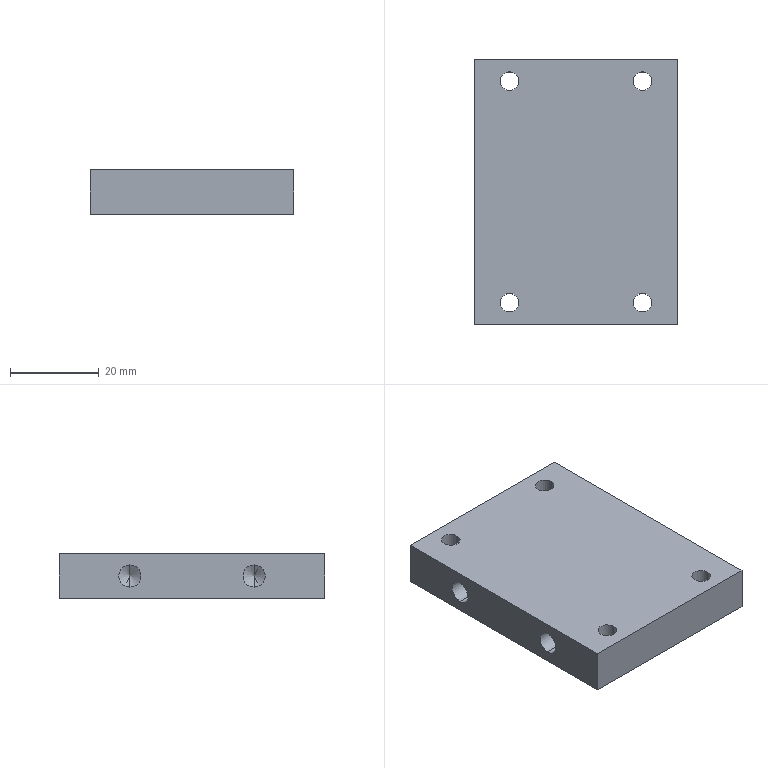Part | 1 solid | 30 faces | box 46 x 60 x 10 mm | volume 25828 mm3 | cylinder 16 | cone 8 | plane 6 | commonest cylinder face diameters 4.2 x8 5 x8
STEP:
#1=CARTESIAN_POINT('',(-17.1,-25.,0.));
#2=VERTEX_POINT('',#1);
#3=CARTESIAN_POINT('',(-12.9,-25.,0.));
#4=VERTEX_POINT('',#3);
#5=CARTESIAN_POINT('',(-15.,-25.,0.));
#6=DIRECTION('',(0.,0.,1.));
#7=DIRECTION('',(1.,0.,0.));
#8=AXIS2_PLACEMENT_3D('',#5,#6,#7);
#9=CIRCLE('',#8,2.1);
#10=EDGE_CURVE('',#2,#4,#9,.T.);
#11=ORIENTED_EDGE('',*,*,#10,.F.);
#12=CARTESIAN_POINT('',(-17.1,-25.,10.));
#13=VERTEX_POINT('',#12);
#14=CARTESIAN_POINT('',(-17.1,-25.,10.));
#15=DIRECTION('',(0.,0.,1.));
#16=VECTOR('',#15,1000.);
#17=LINE('',#14,#16);
#18=EDGE_CURVE('',#2,#13,#17,.T.);
#19=ORIENTED_EDGE('',*,*,#18,.T.);
#20=CARTESIAN_POINT('',(-12.9,-25.,10.));
#21=VERTEX_POINT('',#20);
#22=CARTESIAN_POINT('',(-15.,-25.,10.));
#23=DIRECTION('',(0.,0.,1.));
#24=DIRECTION('',(1.,0.,0.));
#25=AXIS2_PLACEMENT_3D('',#22,#23,#24);
#26=CIRCLE('',#25,2.1);
#27=EDGE_CURVE('',#13,#21,#26,.T.);
#28=ORIENTED_EDGE('',*,*,#27,.T.);
#29=CARTESIAN_POINT('',(-12.9,-25.,10.));
#30=DIRECTION('',(0.,0.,1.));
#31=VECTOR('',#30,1000.);
#32=LINE('',#29,#31);
#33=EDGE_CURVE('',#4,#21,#32,.T.);
#34=ORIENTED_EDGE('',*,*,#33,.F.);
#35=EDGE_LOOP('',(#11,#19,#28,#34));
#36=FACE_OUTER_BOUND('',#35,.T.);
#37=CARTESIAN_POINT('',(-15.,-25.,10.));
#38=DIRECTION('',(0.,0.,1.));
#39=DIRECTION('',(1.,0.,0.));
#40=AXIS2_PLACEMENT_3D('',#37,#38,#39);
#41=CYLINDRICAL_SURFACE('',#40,2.1);
#42=ADVANCED_FACE('',(#36),#41,.F.);
#43=CARTESIAN_POINT('',(12.9,-25.,0.));
#44=VERTEX_POINT('',#43);
#45=CARTESIAN_POINT('',(17.1,-25.,0.));
#46=VERTEX_POINT('',#45);
#47=CARTESIAN_POINT('',(15.,-25.,0.));
#48=DIRECTION('',(0.,0.,1.));
#49=DIRECTION('',(1.,0.,0.));
#50=AXIS2_PLACEMENT_3D('',#47,#48,#49);
#51=CIRCLE('',#50,2.1);
#52=EDGE_CURVE('',#44,#46,#51,.T.);
#53=ORIENTED_EDGE('',*,*,#52,.F.);
#54=CARTESIAN_POINT('',(12.9,-25.,10.));
#55=VERTEX_POINT('',#54);
#56=CARTESIAN_POINT('',(12.9,-25.,10.));
#57=DIRECTION('',(0.,0.,1.));
#58=VECTOR('',#57,1000.);
#59=LINE('',#56,#58);
#60=EDGE_CURVE('',#44,#55,#59,.T.);
#61=ORIENTED_EDGE('',*,*,#60,.T.);
#62=CARTESIAN_POINT('',(17.1,-25.,10.));
#63=VERTEX_POINT('',#62);
#64=CARTESIAN_POINT('',(15.,-25.,10.));
#65=DIRECTION('',(0.,0.,1.));
#66=DIRECTION('',(1.,0.,0.));
#67=AXIS2_PLACEMENT_3D('',#64,#65,#66);
#68=CIRCLE('',#67,2.1);
#69=EDGE_CURVE('',#55,#63,#68,.T.);
#70=ORIENTED_EDGE('',*,*,#69,.T.);
#71=CARTESIAN_POINT('',(17.1,-25.,10.));
#72=DIRECTION('',(0.,0.,1.));
#73=VECTOR('',#72,1000.);
#74=LINE('',#71,#73);
#75=EDGE_CURVE('',#46,#63,#74,.T.);
#76=ORIENTED_EDGE('',*,*,#75,.F.);
#77=EDGE_LOOP('',(#53,#61,#70,#76));
#78=FACE_OUTER_BOUND('',#77,.T.);
#79=CARTESIAN_POINT('',(15.,-25.,10.));
#80=DIRECTION('',(0.,0.,1.));
#81=DIRECTION('',(1.,0.,0.));
#82=AXIS2_PLACEMENT_3D('',#79,#80,#81);
#83=CYLINDRICAL_SURFACE('',#82,2.1);
#84=ADVANCED_FACE('',(#78),#83,.F.);
#85=CARTESIAN_POINT('',(-17.1,25.,0.));
#86=VERTEX_POINT('',#85);
#87=CARTESIAN_POINT('',(-12.9,25.,0.));
#88=VERTEX_POINT('',#87);
#89=CARTESIAN_POINT('',(-15.,25.,0.));
#90=DIRECTION('',(0.,0.,1.));
#91=DIRECTION('',(1.,0.,0.));
#92=AXIS2_PLACEMENT_3D('',#89,#90,#91);
#93=CIRCLE('',#92,2.1);
#94=EDGE_CURVE('',#86,#88,#93,.T.);
#95=ORIENTED_EDGE('',*,*,#94,.F.);
#96=CARTESIAN_POINT('',(-17.1,25.,10.));
#97=VERTEX_POINT('',#96);
#98=CARTESIAN_POINT('',(-17.1,25.,10.));
#99=DIRECTION('',(0.,0.,1.));
#100=VECTOR('',#99,1000.);
#101=LINE('',#98,#100);
#102=EDGE_CURVE('',#86,#97,#101,.T.);
#103=ORIENTED_EDGE('',*,*,#102,.T.);
#104=CARTESIAN_POINT('',(-12.9,25.,10.));
#105=VERTEX_POINT('',#104);
#106=CARTESIAN_POINT('',(-15.,25.,10.));
#107=DIRECTION('',(0.,0.,1.));
#108=DIRECTION('',(1.,0.,0.));
#109=AXIS2_PLACEMENT_3D('',#106,#107,#108);
#110=CIRCLE('',#109,2.1);
#111=EDGE_CURVE('',#97,#105,#110,.T.);
#112=ORIENTED_EDGE('',*,*,#111,.T.);
#113=CARTESIAN_POINT('',(-12.9,25.,10.));
#114=DIRECTION('',(0.,0.,1.));
#115=VECTOR('',#114,1000.);
#116=LINE('',#113,#115);
#117=EDGE_CURVE('',#88,#105,#116,.T.);
#118=ORIENTED_EDGE('',*,*,#117,.F.);
#119=EDGE_LOOP('',(#95,#103,#112,#118));
#120=FACE_OUTER_BOUND('',#119,.T.);
#121=CARTESIAN_POINT('',(-15.,25.,10.));
#122=DIRECTION('',(0.,0.,1.));
#123=DIRECTION('',(1.,0.,0.));
#124=AXIS2_PLACEMENT_3D('',#121,#122,#123);
#125=CYLINDRICAL_SURFACE('',#124,2.1);
#126=ADVANCED_FACE('',(#120),#125,.F.);
#127=CARTESIAN_POINT('',(12.9,25.,0.));
#128=VERTEX_POINT('',#127);
#129=CARTESIAN_POINT('',(17.1,25.,0.));
#130=VERTEX_POINT('',#129);
#131=CARTESIAN_POINT('',(15.,25.,0.));
#132=DIRECTION('',(0.,0.,1.));
#133=DIRECTION('',(1.,0.,0.));
#134=AXIS2_PLACEMENT_3D('',#131,#132,#133);
#135=CIRCLE('',#134,2.1);
#136=EDGE_CURVE('',#128,#130,#135,.T.);
#137=ORIENTED_EDGE('',*,*,#136,.F.);
#138=CARTESIAN_POINT('',(12.9,25.,10.));
#139=VERTEX_POINT('',#138);
#140=CARTESIAN_POINT('',(12.9,25.,10.));
#141=DIRECTION('',(0.,0.,1.));
#142=VECTOR('',#141,1000.);
#143=LINE('',#140,#142);
#144=EDGE_CURVE('',#128,#139,#143,.T.);
#145=ORIENTED_EDGE('',*,*,#144,.T.);
#146=CARTESIAN_POINT('',(17.1,25.,10.));
#147=VERTEX_POINT('',#146);
#148=CARTESIAN_POINT('',(15.,25.,10.));
#149=DIRECTION('',(0.,0.,1.));
#150=DIRECTION('',(1.,0.,0.));
#151=AXIS2_PLACEMENT_3D('',#148,#149,#150);
#152=CIRCLE('',#151,2.1);
#153=EDGE_CURVE('',#139,#147,#152,.T.);
#154=ORIENTED_EDGE('',*,*,#153,.T.);
#155=CARTESIAN_POINT('',(17.1,25.,10.));
#156=DIRECTION('',(0.,0.,1.));
#157=VECTOR('',#156,1000.);
#158=LINE('',#155,#157);
#159=EDGE_CURVE('',#130,#147,#158,.T.);
#160=ORIENTED_EDGE('',*,*,#159,.F.);
#161=EDGE_LOOP('',(#137,#145,#154,#160));
#162=FACE_OUTER_BOUND('',#161,.T.);
#163=CARTESIAN_POINT('',(15.,25.,10.));
#164=DIRECTION('',(0.,0.,1.));
#165=DIRECTION('',(1.,0.,0.));
#166=AXIS2_PLACEMENT_3D('',#163,#164,#165);
#167=CYLINDRICAL_SURFACE('',#166,2.1);
#168=ADVANCED_FACE('',(#162),#167,.F.);
#169=CARTESIAN_POINT('',(8.,14.,7.5));
#170=VERTEX_POINT('',#169);
#171=CARTESIAN_POINT('',(8.,14.,2.5));
#172=VERTEX_POINT('',#171);
#173=CARTESIAN_POINT('',(8.,14.,5.));
#174=DIRECTION('',(1.,0.,0.));
#175=DIRECTION('',(0.,0.,-1.));
#176=AXIS2_PLACEMENT_3D('',#173,#174,#175);
#177=CIRCLE('',#176,2.5);
#178=EDGE_CURVE('',#170,#172,#177,.T.);
#179=ORIENTED_EDGE('',*,*,#178,.F.);
#180=CARTESIAN_POINT('',(23.,14.,7.5));
#181=VERTEX_POINT('',#180);
#182=CARTESIAN_POINT('',(23.,14.,7.5));
#183=DIRECTION('',(1.,0.,0.));
#184=VECTOR('',#183,1000.);
#185=LINE('',#182,#184);
#186=EDGE_CURVE('',#170,#181,#185,.T.);
#187=ORIENTED_EDGE('',*,*,#186,.T.);
#188=CARTESIAN_POINT('',(23.,14.,2.5));
#189=VERTEX_POINT('',#188);
#190=CARTESIAN_POINT('',(23.,14.,5.));
#191=DIRECTION('',(1.,0.,0.));
#192=DIRECTION('',(0.,0.,-1.));
#193=AXIS2_PLACEMENT_3D('',#190,#191,#192);
#194=CIRCLE('',#193,2.5);
#195=EDGE_CURVE('',#181,#189,#194,.T.);
#196=ORIENTED_EDGE('',*,*,#195,.T.);
#197=CARTESIAN_POINT('',(23.,14.,2.5));
#198=DIRECTION('',(1.,0.,0.));
#199=VECTOR('',#198,1000.);
#200=LINE('',#197,#199);
#201=EDGE_CURVE('',#172,#189,#200,.T.);
#202=ORIENTED_EDGE('',*,*,#201,.F.);
#203=EDGE_LOOP('',(#179,#187,#196,#202));
#204=FACE_OUTER_BOUND('',#203,.T.);
#205=CARTESIAN_POINT('',(23.,14.,5.));
#206=DIRECTION('',(1.,0.,0.));
#207=DIRECTION('',(0.,0.,-1.));
#208=AXIS2_PLACEMENT_3D('',#205,#206,#207);
#209=CYLINDRICAL_SURFACE('',#208,2.5);
#210=ADVANCED_FACE('',(#204),#209,.F.);
#211=CARTESIAN_POINT('',(6.498,14.,5.));
#212=VERTEX_POINT('',#211);
#213=CARTESIAN_POINT('',(8.,14.,2.5));
#214=DIRECTION('',(0.515,0.,-0.8572));
#215=VECTOR('',#214,1000.);
#216=LINE('',#213,#215);
#217=EDGE_CURVE('',#212,#172,#216,.T.);
#218=ORIENTED_EDGE('',*,*,#217,.F.);
#219=CARTESIAN_POINT('',(8.,14.,7.5));
#220=DIRECTION('',(0.515,0.,0.8572));
#221=VECTOR('',#220,1000.);
#222=LINE('',#219,#221);
#223=EDGE_CURVE('',#212,#170,#222,.T.);
#224=ORIENTED_EDGE('',*,*,#223,.T.);
#225=ORIENTED_EDGE('',*,*,#178,.T.);
#226=EDGE_LOOP('',(#218,#224,#225));
#227=FACE_OUTER_BOUND('',#226,.T.);
#228=CARTESIAN_POINT('',(8.,14.,5.));
#229=DIRECTION('',(1.,0.,0.));
#230=DIRECTION('',(0.,0.,-1.));
#231=AXIS2_PLACEMENT_3D('',#228,#229,#230);
#232=CONICAL_SURFACE('',#231,2.5,1.03);
#233=ADVANCED_FACE('',(#227),#232,.F.);
#234=CARTESIAN_POINT('',(8.,-14.,7.5));
#235=VERTEX_POINT('',#234);
#236=CARTESIAN_POINT('',(8.,-14.,2.5));
#237=VERTEX_POINT('',#236);
#238=CARTESIAN_POINT('',(8.,-14.,5.));
#239=DIRECTION('',(1.,0.,0.));
#240=DIRECTION('',(0.,0.,-1.));
#241=AXIS2_PLACEMENT_3D('',#238,#239,#240);
#242=CIRCLE('',#241,2.5);
#243=EDGE_CURVE('',#235,#237,#242,.T.);
#244=ORIENTED_EDGE('',*,*,#243,.F.);
#245=CARTESIAN_POINT('',(23.,-14.,7.5));
#246=VERTEX_POINT('',#245);
#247=CARTESIAN_POINT('',(23.,-14.,7.5));
#248=DIRECTION('',(1.,0.,0.));
#249=VECTOR('',#248,1000.);
#250=LINE('',#247,#249);
#251=EDGE_CURVE('',#235,#246,#250,.T.);
#252=ORIENTED_EDGE('',*,*,#251,.T.);
#253=CARTESIAN_POINT('',(23.,-14.,2.5));
#254=VERTEX_POINT('',#253);
#255=CARTESIAN_POINT('',(23.,-14.,5.));
#256=DIRECTION('',(1.,0.,0.));
#257=DIRECTION('',(0.,0.,-1.));
#258=AXIS2_PLACEMENT_3D('',#255,#256,#257);
#259=CIRCLE('',#258,2.5);
#260=EDGE_CURVE('',#246,#254,#259,.T.);
#261=ORIENTED_EDGE('',*,*,#260,.T.);
#262=CARTESIAN_POINT('',(23.,-14.,2.5));
#263=DIRECTION('',(1.,0.,0.));
#264=VECTOR('',#263,1000.);
#265=LINE('',#262,#264);
#266=EDGE_CURVE('',#237,#254,#265,.T.);
#267=ORIENTED_EDGE('',*,*,#266,.F.);
#268=EDGE_LOOP('',(#244,#252,#261,#267));
#269=FACE_OUTER_BOUND('',#268,.T.);
#270=CARTESIAN_POINT('',(23.,-14.,5.));
#271=DIRECTION('',(1.,0.,0.));
#272=DIRECTION('',(0.,0.,-1.));
#273=AXIS2_PLACEMENT_3D('',#270,#271,#272);
#274=CYLINDRICAL_SURFACE('',#273,2.5);
#275=ADVANCED_FACE('',(#269),#274,.F.);
#276=CARTESIAN_POINT('',(6.498,-14.,5.));
#277=VERTEX_POINT('',#276);
#278=CARTESIAN_POINT('',(8.,-14.,2.5));
#279=DIRECTION('',(0.515,0.,-0.8572));
#280=VECTOR('',#279,1000.);
#281=LINE('',#278,#280);
#282=EDGE_CURVE('',#277,#237,#281,.T.);
#283=ORIENTED_EDGE('',*,*,#282,.F.);
#284=CARTESIAN_POINT('',(8.,-14.,7.5));
#285=DIRECTION('',(0.515,0.,0.8572));
#286=VECTOR('',#285,1000.);
#287=LINE('',#284,#286);
#288=EDGE_CURVE('',#277,#235,#287,.T.);
#289=ORIENTED_EDGE('',*,*,#288,.T.);
#290=ORIENTED_EDGE('',*,*,#243,.T.);
#291=EDGE_LOOP('',(#283,#289,#290));
#292=FACE_OUTER_BOUND('',#291,.T.);
#293=CARTESIAN_POINT('',(8.,-14.,5.));
#294=DIRECTION('',(1.,0.,0.));
#295=DIRECTION('',(0.,0.,-1.));
#296=AXIS2_PLACEMENT_3D('',#293,#294,#295);
#297=CONICAL_SURFACE('',#296,2.5,1.03);
#298=ADVANCED_FACE('',(#292),#297,.F.);
#299=CARTESIAN_POINT('',(-8.,14.,2.5));
#300=VERTEX_POINT('',#299);
#301=CARTESIAN_POINT('',(-8.,14.,7.5));
#302=VERTEX_POINT('',#301);
#303=CARTESIAN_POINT('',(-8.,14.,5.));
#304=DIRECTION('',(-1.,0.,0.));
#305=DIRECTION('',(0.,0.,1.));
#306=AXIS2_PLACEMENT_3D('',#303,#304,#305);
#307=CIRCLE('',#306,2.5);
#308=EDGE_CURVE('',#300,#302,#307,.T.);
#309=ORIENTED_EDGE('',*,*,#308,.F.);
#310=CARTESIAN_POINT('',(-23.,14.,2.5));
#311=VERTEX_POINT('',#310);
#312=CARTESIAN_POINT('',(-23.,14.,2.5));
#313=DIRECTION('',(-1.,0.,0.));
#314=VECTOR('',#313,1000.);
#315=LINE('',#312,#314);
#316=EDGE_CURVE('',#300,#311,#315,.T.);
#317=ORIENTED_EDGE('',*,*,#316,.T.);
#318=CARTESIAN_POINT('',(-23.,14.,7.5));
#319=VERTEX_POINT('',#318);
#320=CARTESIAN_POINT('',(-23.,14.,5.));
#321=DIRECTION('',(-1.,0.,0.));
#322=DIRECTION('',(0.,0.,1.));
#323=AXIS2_PLACEMENT_3D('',#320,#321,#322);
#324=CIRCLE('',#323,2.5);
#325=EDGE_CURVE('',#311,#319,#324,.T.);
#326=ORIENTED_EDGE('',*,*,#325,.T.);
#327=CARTESIAN_POINT('',(-23.,14.,7.5));
#328=DIRECTION('',(-1.,0.,0.));
#329=VECTOR('',#328,1000.);
#330=LINE('',#327,#329);
#331=EDGE_CURVE('',#302,#319,#330,.T.);
#332=ORIENTED_EDGE('',*,*,#331,.F.);
#333=EDGE_LOOP('',(#309,#317,#326,#332));
#334=FACE_OUTER_BOUND('',#333,.T.);
#335=CARTESIAN_POINT('',(-23.,14.,5.));
#336=DIRECTION('',(-1.,0.,0.));
#337=DIRECTION('',(0.,0.,1.));
#338=AXIS2_PLACEMENT_3D('',#335,#336,#337);
#339=CYLINDRICAL_SURFACE('',#338,2.5);
#340=ADVANCED_FACE('',(#334),#339,.F.);
#341=CARTESIAN_POINT('',(-6.498,14.,5.));
#342=VERTEX_POINT('',#341);
#343=CARTESIAN_POINT('',(-8.,14.,7.5));
#344=DIRECTION('',(-0.515,0.,0.8572));
#345=VECTOR('',#344,1000.);
#346=LINE('',#343,#345);
#347=EDGE_CURVE('',#342,#302,#346,.T.);
#348=ORIENTED_EDGE('',*,*,#347,.F.);
#349=CARTESIAN_POINT('',(-8.,14.,2.5));
#350=DIRECTION('',(-0.515,0.,-0.8572));
#351=VECTOR('',#350,1000.);
#352=LINE('',#349,#351);
#353=EDGE_CURVE('',#342,#300,#352,.T.);
#354=ORIENTED_EDGE('',*,*,#353,.T.);
#355=ORIENTED_EDGE('',*,*,#308,.T.);
#356=EDGE_LOOP('',(#348,#354,#355));
#357=FACE_OUTER_BOUND('',#356,.T.);
#358=CARTESIAN_POINT('',(-8.,14.,5.));
#359=DIRECTION('',(-1.,0.,0.));
#360=DIRECTION('',(0.,0.,1.));
#361=AXIS2_PLACEMENT_3D('',#358,#359,#360);
#362=CONICAL_SURFACE('',#361,2.5,1.03);
#363=ADVANCED_FACE('',(#357),#362,.F.);
#364=CARTESIAN_POINT('',(-8.,-14.,2.5));
#365=VERTEX_POINT('',#364);
#366=CARTESIAN_POINT('',(-8.,-14.,7.5));
#367=VERTEX_POINT('',#366);
#368=CARTESIAN_POINT('',(-8.,-14.,5.));
#369=DIRECTION('',(-1.,0.,0.));
#370=DIRECTION('',(0.,0.,1.));
#371=AXIS2_PLACEMENT_3D('',#368,#369,#370);
#372=CIRCLE('',#371,2.5);
#373=EDGE_CURVE('',#365,#367,#372,.T.);
#374=ORIENTED_EDGE('',*,*,#373,.F.);
#375=CARTESIAN_POINT('',(-23.,-14.,2.5));
#376=VERTEX_POINT('',#375);
#377=CARTESIAN_POINT('',(-23.,-14.,2.5));
#378=DIRECTION('',(-1.,0.,0.));
#379=VECTOR('',#378,1000.);
#380=LINE('',#377,#379);
#381=EDGE_CURVE('',#365,#376,#380,.T.);
#382=ORIENTED_EDGE('',*,*,#381,.T.);
#383=CARTESIAN_POINT('',(-23.,-14.,7.5));
#384=VERTEX_POINT('',#383);
#385=CARTESIAN_POINT('',(-23.,-14.,5.));
#386=DIRECTION('',(-1.,0.,0.));
#387=DIRECTION('',(0.,0.,1.));
#388=AXIS2_PLACEMENT_3D('',#385,#386,#387);
#389=CIRCLE('',#388,2.5);
#390=EDGE_CURVE('',#376,#384,#389,.T.);
#391=ORIENTED_EDGE('',*,*,#390,.T.);
#392=CARTESIAN_POINT('',(-23.,-14.,7.5));
#393=DIRECTION('',(-1.,0.,0.));
#394=VECTOR('',#393,1000.);
#395=LINE('',#392,#394);
#396=EDGE_CURVE('',#367,#384,#395,.T.);
#397=ORIENTED_EDGE('',*,*,#396,.F.);
#398=EDGE_LOOP('',(#374,#382,#391,#397));
#399=FACE_OUTER_BOUND('',#398,.T.);
#400=CARTESIAN_POINT('',(-23.,-14.,5.));
#401=DIRECTION('',(-1.,0.,0.));
#402=DIRECTION('',(0.,0.,1.));
#403=AXIS2_PLACEMENT_3D('',#400,#401,#402);
#404=CYLINDRICAL_SURFACE('',#403,2.5);
#405=ADVANCED_FACE('',(#399),#404,.F.);
#406=CARTESIAN_POINT('',(-6.498,-14.,5.));
#407=VERTEX_POINT('',#406);
#408=CARTESIAN_POINT('',(-8.,-14.,7.5));
#409=DIRECTION('',(-0.515,0.,0.8572));
#410=VECTOR('',#409,1000.);
#411=LINE('',#408,#410);
#412=EDGE_CURVE('',#407,#367,#411,.T.);
#413=ORIENTED_EDGE('',*,*,#412,.F.);
#414=CARTESIAN_POINT('',(-8.,-14.,2.5));
#415=DIRECTION('',(-0.515,0.,-0.8572));
#416=VECTOR('',#415,1000.);
#417=LINE('',#414,#416);
#418=EDGE_CURVE('',#407,#365,#417,.T.);
#419=ORIENTED_EDGE('',*,*,#418,.T.);
#420=ORIENTED_EDGE('',*,*,#373,.T.);
#421=EDGE_LOOP('',(#413,#419,#420));
#422=FACE_OUTER_BOUND('',#421,.T.);
#423=CARTESIAN_POINT('',(-8.,-14.,5.));
#424=DIRECTION('',(-1.,0.,0.));
#425=DIRECTION('',(0.,0.,1.));
#426=AXIS2_PLACEMENT_3D('',#423,#424,#425);
#427=CONICAL_SURFACE('',#426,2.5,1.03);
#428=ADVANCED_FACE('',(#422),#427,.F.);
#429=CARTESIAN_POINT('',(-15.,-25.,10.));
#430=DIRECTION('',(0.,0.,1.));
#431=DIRECTION('',(1.,0.,0.));
#432=AXIS2_PLACEMENT_3D('',#429,#430,#431);
#433=CIRCLE('',#432,2.1);
#434=EDGE_CURVE('',#21,#13,#433,.T.);
#435=ORIENTED_EDGE('',*,*,#434,.F.);
#436=ORIENTED_EDGE('',*,*,#27,.F.);
#437=EDGE_LOOP('',(#435,#436));
#438=FACE_BOUND('',#437,.T.);
#439=CARTESIAN_POINT('',(15.,-25.,10.));
#440=DIRECTION('',(0.,0.,1.));
#441=DIRECTION('',(1.,0.,0.));
#442=AXIS2_PLACEMENT_3D('',#439,#440,#441);
#443=CIRCLE('',#442,2.1);
#444=EDGE_CURVE('',#63,#55,#443,.T.);
#445=ORIENTED_EDGE('',*,*,#444,.F.);
#446=ORIENTED_EDGE('',*,*,#69,.F.);
#447=EDGE_LOOP('',(#445,#446));
#448=FACE_BOUND('',#447,.T.);
#449=CARTESIAN_POINT('',(-15.,25.,10.));
#450=DIRECTION('',(0.,0.,1.));
#451=DIRECTION('',(1.,0.,0.));
#452=AXIS2_PLACEMENT_3D('',#449,#450,#451);
#453=CIRCLE('',#452,2.1);
#454=EDGE_CURVE('',#105,#97,#453,.T.);
#455=ORIENTED_EDGE('',*,*,#454,.F.);
#456=ORIENTED_EDGE('',*,*,#111,.F.);
#457=EDGE_LOOP('',(#455,#456));
#458=FACE_BOUND('',#457,.T.);
#459=CARTESIAN_POINT('',(23.,-30.,10.));
#460=VERTEX_POINT('',#459);
#461=CARTESIAN_POINT('',(23.,30.,10.));
#462=VERTEX_POINT('',#461);
#463=CARTESIAN_POINT('',(23.,-30.,10.));
#464=DIRECTION('',(0.,1.,0.));
#465=VECTOR('',#464,1000.);
#466=LINE('',#463,#465);
#467=EDGE_CURVE('',#460,#462,#466,.T.);
#468=ORIENTED_EDGE('',*,*,#467,.T.);
#469=CARTESIAN_POINT('',(-23.,30.,10.));
#470=VERTEX_POINT('',#469);
#471=CARTESIAN_POINT('',(-23.,30.,10.));
#472=DIRECTION('',(-1.,0.,0.));
#473=VECTOR('',#472,1000.);
#474=LINE('',#471,#473);
#475=EDGE_CURVE('',#462,#470,#474,.T.);
#476=ORIENTED_EDGE('',*,*,#475,.T.);
#477=CARTESIAN_POINT('',(-23.,-30.,10.));
#478=VERTEX_POINT('',#477);
#479=CARTESIAN_POINT('',(-23.,-30.,10.));
#480=DIRECTION('',(0.,-1.,0.));
#481=VECTOR('',#480,1000.);
#482=LINE('',#479,#481);
#483=EDGE_CURVE('',#470,#478,#482,.T.);
#484=ORIENTED_EDGE('',*,*,#483,.T.);
#485=CARTESIAN_POINT('',(-23.,-30.,10.));
#486=DIRECTION('',(1.,0.,0.));
#487=VECTOR('',#486,1000.);
#488=LINE('',#485,#487);
#489=EDGE_CURVE('',#478,#460,#488,.T.);
#490=ORIENTED_EDGE('',*,*,#489,.T.);
#491=EDGE_LOOP('',(#468,#476,#484,#490));
#492=FACE_OUTER_BOUND('',#491,.T.);
#493=CARTESIAN_POINT('',(15.,25.,10.));
#494=DIRECTION('',(0.,0.,1.));
#495=DIRECTION('',(1.,0.,0.));
#496=AXIS2_PLACEMENT_3D('',#493,#494,#495);
#497=CIRCLE('',#496,2.1);
#498=EDGE_CURVE('',#147,#139,#497,.T.);
#499=ORIENTED_EDGE('',*,*,#498,.F.);
#500=ORIENTED_EDGE('',*,*,#153,.F.);
#501=EDGE_LOOP('',(#499,#500));
#502=FACE_BOUND('',#501,.T.);
#503=CARTESIAN_POINT('',(0.,0.,10.));
#504=DIRECTION('',(0.,0.,-1.));
#505=DIRECTION('',(-1.,0.,0.));
#506=AXIS2_PLACEMENT_3D('',#503,#504,#505);
#507=PLANE('',#506);
#508=ADVANCED_FACE('',(#438,#448,#458,#492,#502),#507,.F.);
#509=CARTESIAN_POINT('',(-15.,-25.,0.));
#510=DIRECTION('',(0.,0.,1.));
#511=DIRECTION('',(1.,0.,0.));
#512=AXIS2_PLACEMENT_3D('',#509,#510,#511);
#513=CIRCLE('',#512,2.1);
#514=EDGE_CURVE('',#4,#2,#513,.T.);
#515=ORIENTED_EDGE('',*,*,#514,.T.);
#516=ORIENTED_EDGE('',*,*,#10,.T.);
#517=EDGE_LOOP('',(#515,#516));
#518=FACE_BOUND('',#517,.T.);
#519=CARTESIAN_POINT('',(15.,-25.,0.));
#520=DIRECTION('',(0.,0.,1.));
#521=DIRECTION('',(1.,0.,0.));
#522=AXIS2_PLACEMENT_3D('',#519,#520,#521);
#523=CIRCLE('',#522,2.1);
#524=EDGE_CURVE('',#46,#44,#523,.T.);
#525=ORIENTED_EDGE('',*,*,#524,.T.);
#526=ORIENTED_EDGE('',*,*,#52,.T.);
#527=EDGE_LOOP('',(#525,#526));
#528=FACE_BOUND('',#527,.T.);
#529=CARTESIAN_POINT('',(-15.,25.,0.));
#530=DIRECTION('',(0.,0.,1.));
#531=DIRECTION('',(1.,0.,0.));
#532=AXIS2_PLACEMENT_3D('',#529,#530,#531);
#533=CIRCLE('',#532,2.1);
#534=EDGE_CURVE('',#88,#86,#533,.T.);
#535=ORIENTED_EDGE('',*,*,#534,.T.);
#536=ORIENTED_EDGE('',*,*,#94,.T.);
#537=EDGE_LOOP('',(#535,#536));
#538=FACE_BOUND('',#537,.T.);
#539=CARTESIAN_POINT('',(23.,-30.,0.));
#540=VERTEX_POINT('',#539);
#541=CARTESIAN_POINT('',(23.,30.,0.));
#542=VERTEX_POINT('',#541);
#543=CARTESIAN_POINT('',(23.,-30.,0.));
#544=DIRECTION('',(0.,1.,0.));
#545=VECTOR('',#544,1000.);
#546=LINE('',#543,#545);
#547=EDGE_CURVE('',#540,#542,#546,.T.);
#548=ORIENTED_EDGE('',*,*,#547,.F.);
#549=CARTESIAN_POINT('',(-23.,-30.,0.));
#550=VERTEX_POINT('',#549);
#551=CARTESIAN_POINT('',(-23.,-30.,0.));
#552=DIRECTION('',(1.,0.,0.));
#553=VECTOR('',#552,1000.);
#554=LINE('',#551,#553);
#555=EDGE_CURVE('',#550,#540,#554,.T.);
#556=ORIENTED_EDGE('',*,*,#555,.F.);
#557=CARTESIAN_POINT('',(-23.,30.,0.));
#558=VERTEX_POINT('',#557);
#559=CARTESIAN_POINT('',(-23.,-30.,0.));
#560=DIRECTION('',(0.,-1.,0.));
#561=VECTOR('',#560,1000.);
#562=LINE('',#559,#561);
#563=EDGE_CURVE('',#558,#550,#562,.T.);
#564=ORIENTED_EDGE('',*,*,#563,.F.);
#565=CARTESIAN_POINT('',(-23.,30.,0.));
#566=DIRECTION('',(-1.,0.,0.));
#567=VECTOR('',#566,1000.);
#568=LINE('',#565,#567);
#569=EDGE_CURVE('',#542,#558,#568,.T.);
#570=ORIENTED_EDGE('',*,*,#569,.F.);
#571=EDGE_LOOP('',(#548,#556,#564,#570));
#572=FACE_OUTER_BOUND('',#571,.T.);
#573=CARTESIAN_POINT('',(15.,25.,0.));
#574=DIRECTION('',(0.,0.,1.));
#575=DIRECTION('',(1.,0.,0.));
#576=AXIS2_PLACEMENT_3D('',#573,#574,#575);
#577=CIRCLE('',#576,2.1);
#578=EDGE_CURVE('',#130,#128,#577,.T.);
#579=ORIENTED_EDGE('',*,*,#578,.T.);
#580=ORIENTED_EDGE('',*,*,#136,.T.);
#581=EDGE_LOOP('',(#579,#580));
#582=FACE_BOUND('',#581,.T.);
#583=CARTESIAN_POINT('',(0.,0.,0.));
#584=DIRECTION('',(0.,0.,-1.));
#585=DIRECTION('',(-1.,0.,0.));
#586=AXIS2_PLACEMENT_3D('',#583,#584,#585);
#587=PLANE('',#586);
#588=ADVANCED_FACE('',(#518,#528,#538,#572,#582),#587,.T.);
#589=CARTESIAN_POINT('',(23.,14.,5.));
#590=DIRECTION('',(1.,0.,0.));
#591=DIRECTION('',(0.,0.,-1.));
#592=AXIS2_PLACEMENT_3D('',#589,#590,#591);
#593=CIRCLE('',#592,2.5);
#594=EDGE_CURVE('',#189,#181,#593,.T.);
#595=ORIENTED_EDGE('',*,*,#594,.F.);
#596=ORIENTED_EDGE('',*,*,#195,.F.);
#597=EDGE_LOOP('',(#595,#596));
#598=FACE_BOUND('',#597,.T.);
#599=CARTESIAN_POINT('',(23.,-14.,5.));
#600=DIRECTION('',(1.,0.,0.));
#601=DIRECTION('',(0.,0.,-1.));
#602=AXIS2_PLACEMENT_3D('',#599,#600,#601);
#603=CIRCLE('',#602,2.5);
#604=EDGE_CURVE('',#254,#246,#603,.T.);
#605=ORIENTED_EDGE('',*,*,#604,.F.);
#606=ORIENTED_EDGE('',*,*,#260,.F.);
#607=EDGE_LOOP('',(#605,#606));
#608=FACE_BOUND('',#607,.T.);
#609=ORIENTED_EDGE('',*,*,#547,.T.);
#610=CARTESIAN_POINT('',(23.,30.,10.));
#611=DIRECTION('',(0.,0.,-1.));
#612=VECTOR('',#611,1000.);
#613=LINE('',#610,#612);
#614=EDGE_CURVE('',#462,#542,#613,.T.);
#615=ORIENTED_EDGE('',*,*,#614,.F.);
#616=ORIENTED_EDGE('',*,*,#467,.F.);
#617=CARTESIAN_POINT('',(23.,-30.,10.));
#618=DIRECTION('',(0.,0.,-1.));
#619=VECTOR('',#618,1000.);
#620=LINE('',#617,#619);
#621=EDGE_CURVE('',#460,#540,#620,.T.);
#622=ORIENTED_EDGE('',*,*,#621,.T.);
#623=EDGE_LOOP('',(#609,#615,#616,#622));
#624=FACE_OUTER_BOUND('',#623,.T.);
#625=CARTESIAN_POINT('',(23.,-30.,10.));
#626=DIRECTION('',(-1.,0.,0.));
#627=DIRECTION('',(0.,-1.,0.));
#628=AXIS2_PLACEMENT_3D('',#625,#626,#627);
#629=PLANE('',#628);
#630=ADVANCED_FACE('',(#598,#608,#624),#629,.F.);
#631=ORIENTED_EDGE('',*,*,#569,.T.);
#632=CARTESIAN_POINT('',(-23.,30.,10.));
#633=DIRECTION('',(0.,0.,-1.));
#634=VECTOR('',#633,1000.);
#635=LINE('',#632,#634);
#636=EDGE_CURVE('',#470,#558,#635,.T.);
#637=ORIENTED_EDGE('',*,*,#636,.F.);
#638=ORIENTED_EDGE('',*,*,#475,.F.);
#639=ORIENTED_EDGE('',*,*,#614,.T.);
#640=EDGE_LOOP('',(#631,#637,#638,#639));
#641=FACE_OUTER_BOUND('',#640,.T.);
#642=CARTESIAN_POINT('',(-23.,30.,10.));
#643=DIRECTION('',(0.,-1.,0.));
#644=DIRECTION('',(1.,0.,0.));
#645=AXIS2_PLACEMENT_3D('',#642,#643,#644);
#646=PLANE('',#645);
#647=ADVANCED_FACE('',(#641),#646,.F.);
#648=CARTESIAN_POINT('',(-23.,14.,5.));
#649=DIRECTION('',(-1.,0.,0.));
#650=DIRECTION('',(0.,0.,1.));
#651=AXIS2_PLACEMENT_3D('',#648,#649,#650);
#652=CIRCLE('',#651,2.5);
#653=EDGE_CURVE('',#319,#311,#652,.T.);
#654=ORIENTED_EDGE('',*,*,#653,.F.);
#655=ORIENTED_EDGE('',*,*,#325,.F.);
#656=EDGE_LOOP('',(#654,#655));
#657=FACE_BOUND('',#656,.T.);
#658=CARTESIAN_POINT('',(-23.,-14.,5.));
#659=DIRECTION('',(-1.,0.,0.));
#660=DIRECTION('',(0.,0.,1.));
#661=AXIS2_PLACEMENT_3D('',#658,#659,#660);
#662=CIRCLE('',#661,2.5);
#663=EDGE_CURVE('',#384,#376,#662,.T.);
#664=ORIENTED_EDGE('',*,*,#663,.F.);
#665=ORIENTED_EDGE('',*,*,#390,.F.);
#666=EDGE_LOOP('',(#664,#665));
#667=FACE_BOUND('',#666,.T.);
#668=ORIENTED_EDGE('',*,*,#563,.T.);
#669=CARTESIAN_POINT('',(-23.,-30.,10.));
#670=DIRECTION('',(0.,0.,-1.));
#671=VECTOR('',#670,1000.);
#672=LINE('',#669,#671);
#673=EDGE_CURVE('',#478,#550,#672,.T.);
#674=ORIENTED_EDGE('',*,*,#673,.F.);
#675=ORIENTED_EDGE('',*,*,#483,.F.);
#676=ORIENTED_EDGE('',*,*,#636,.T.);
#677=EDGE_LOOP('',(#668,#674,#675,#676));
#678=FACE_OUTER_BOUND('',#677,.T.);
#679=CARTESIAN_POINT('',(-23.,-30.,10.));
#680=DIRECTION('',(1.,0.,0.));
#681=DIRECTION('',(0.,1.,0.));
#682=AXIS2_PLACEMENT_3D('',#679,#680,#681);
#683=PLANE('',#682);
#684=ADVANCED_FACE('',(#657,#667,#678),#683,.F.);
#685=ORIENTED_EDGE('',*,*,#555,.T.);
#686=ORIENTED_EDGE('',*,*,#621,.F.);
#687=ORIENTED_EDGE('',*,*,#489,.F.);
#688=ORIENTED_EDGE('',*,*,#673,.T.);
#689=EDGE_LOOP('',(#685,#686,#687,#688));
#690=FACE_OUTER_BOUND('',#689,.T.);
#691=CARTESIAN_POINT('',(-23.,-30.,10.));
#692=DIRECTION('',(0.,1.,0.));
#693=DIRECTION('',(-1.,0.,0.));
#694=AXIS2_PLACEMENT_3D('',#691,#692,#693);
#695=PLANE('',#694);
#696=ADVANCED_FACE('',(#690),#695,.F.);
#697=ORIENTED_EDGE('',*,*,#418,.F.);
#698=ORIENTED_EDGE('',*,*,#412,.T.);
#699=CARTESIAN_POINT('',(-8.,-14.,5.));
#700=DIRECTION('',(-1.,0.,0.));
#701=DIRECTION('',(0.,0.,1.));
#702=AXIS2_PLACEMENT_3D('',#699,#700,#701);
#703=CIRCLE('',#702,2.5);
#704=EDGE_CURVE('',#367,#365,#703,.T.);
#705=ORIENTED_EDGE('',*,*,#704,.T.);
#706=EDGE_LOOP('',(#697,#698,#705));
#707=FACE_OUTER_BOUND('',#706,.T.);
#708=CARTESIAN_POINT('',(-8.,-14.,5.));
#709=DIRECTION('',(-1.,0.,0.));
#710=DIRECTION('',(0.,0.,1.));
#711=AXIS2_PLACEMENT_3D('',#708,#709,#710);
#712=CONICAL_SURFACE('',#711,2.5,1.03);
#713=ADVANCED_FACE('',(#707),#712,.F.);
#714=ORIENTED_EDGE('',*,*,#381,.F.);
#715=ORIENTED_EDGE('',*,*,#704,.F.);
#716=ORIENTED_EDGE('',*,*,#396,.T.);
#717=ORIENTED_EDGE('',*,*,#663,.T.);
#718=EDGE_LOOP('',(#714,#715,#716,#717));
#719=FACE_OUTER_BOUND('',#718,.T.);
#720=CARTESIAN_POINT('',(-23.,-14.,5.));
#721=DIRECTION('',(-1.,0.,0.));
#722=DIRECTION('',(0.,0.,1.));
#723=AXIS2_PLACEMENT_3D('',#720,#721,#722);
#724=CYLINDRICAL_SURFACE('',#723,2.5);
#725=ADVANCED_FACE('',(#719),#724,.F.);
#726=ORIENTED_EDGE('',*,*,#353,.F.);
#727=ORIENTED_EDGE('',*,*,#347,.T.);
#728=CARTESIAN_POINT('',(-8.,14.,5.));
#729=DIRECTION('',(-1.,0.,0.));
#730=DIRECTION('',(0.,0.,1.));
#731=AXIS2_PLACEMENT_3D('',#728,#729,#730);
#732=CIRCLE('',#731,2.5);
#733=EDGE_CURVE('',#302,#300,#732,.T.);
#734=ORIENTED_EDGE('',*,*,#733,.T.);
#735=EDGE_LOOP('',(#726,#727,#734));
#736=FACE_OUTER_BOUND('',#735,.T.);
#737=CARTESIAN_POINT('',(-8.,14.,5.));
#738=DIRECTION('',(-1.,0.,0.));
#739=DIRECTION('',(0.,0.,1.));
#740=AXIS2_PLACEMENT_3D('',#737,#738,#739);
#741=CONICAL_SURFACE('',#740,2.5,1.03);
#742=ADVANCED_FACE('',(#736),#741,.F.);
#743=ORIENTED_EDGE('',*,*,#316,.F.);
#744=ORIENTED_EDGE('',*,*,#733,.F.);
#745=ORIENTED_EDGE('',*,*,#331,.T.);
#746=ORIENTED_EDGE('',*,*,#653,.T.);
#747=EDGE_LOOP('',(#743,#744,#745,#746));
#748=FACE_OUTER_BOUND('',#747,.T.);
#749=CARTESIAN_POINT('',(-23.,14.,5.));
#750=DIRECTION('',(-1.,0.,0.));
#751=DIRECTION('',(0.,0.,1.));
#752=AXIS2_PLACEMENT_3D('',#749,#750,#751);
#753=CYLINDRICAL_SURFACE('',#752,2.5);
#754=ADVANCED_FACE('',(#748),#753,.F.);
#755=ORIENTED_EDGE('',*,*,#288,.F.);
#756=ORIENTED_EDGE('',*,*,#282,.T.);
#757=CARTESIAN_POINT('',(8.,-14.,5.));
#758=DIRECTION('',(1.,0.,0.));
#759=DIRECTION('',(0.,0.,-1.));
#760=AXIS2_PLACEMENT_3D('',#757,#758,#759);
#761=CIRCLE('',#760,2.5);
#762=EDGE_CURVE('',#237,#235,#761,.T.);
#763=ORIENTED_EDGE('',*,*,#762,.T.);
#764=EDGE_LOOP('',(#755,#756,#763));
#765=FACE_OUTER_BOUND('',#764,.T.);
#766=CARTESIAN_POINT('',(8.,-14.,5.));
#767=DIRECTION('',(1.,0.,0.));
#768=DIRECTION('',(0.,0.,-1.));
#769=AXIS2_PLACEMENT_3D('',#766,#767,#768);
#770=CONICAL_SURFACE('',#769,2.5,1.03);
#771=ADVANCED_FACE('',(#765),#770,.F.);
#772=ORIENTED_EDGE('',*,*,#251,.F.);
#773=ORIENTED_EDGE('',*,*,#762,.F.);
#774=ORIENTED_EDGE('',*,*,#266,.T.);
#775=ORIENTED_EDGE('',*,*,#604,.T.);
#776=EDGE_LOOP('',(#772,#773,#774,#775));
#777=FACE_OUTER_BOUND('',#776,.T.);
#778=CARTESIAN_POINT('',(23.,-14.,5.));
#779=DIRECTION('',(1.,0.,0.));
#780=DIRECTION('',(0.,0.,-1.));
#781=AXIS2_PLACEMENT_3D('',#778,#779,#780);
#782=CYLINDRICAL_SURFACE('',#781,2.5);
#783=ADVANCED_FACE('',(#777),#782,.F.);
#784=ORIENTED_EDGE('',*,*,#223,.F.);
#785=ORIENTED_EDGE('',*,*,#217,.T.);
#786=CARTESIAN_POINT('',(8.,14.,5.));
#787=DIRECTION('',(1.,0.,0.));
#788=DIRECTION('',(0.,0.,-1.));
#789=AXIS2_PLACEMENT_3D('',#786,#787,#788);
#790=CIRCLE('',#789,2.5);
#791=EDGE_CURVE('',#172,#170,#790,.T.);
#792=ORIENTED_EDGE('',*,*,#791,.T.);
#793=EDGE_LOOP('',(#784,#785,#792));
#794=FACE_OUTER_BOUND('',#793,.T.);
#795=CARTESIAN_POINT('',(8.,14.,5.));
#796=DIRECTION('',(1.,0.,0.));
#797=DIRECTION('',(0.,0.,-1.));
#798=AXIS2_PLACEMENT_3D('',#795,#796,#797);
#799=CONICAL_SURFACE('',#798,2.5,1.03);
#800=ADVANCED_FACE('',(#794),#799,.F.);
#801=ORIENTED_EDGE('',*,*,#186,.F.);
#802=ORIENTED_EDGE('',*,*,#791,.F.);
#803=ORIENTED_EDGE('',*,*,#201,.T.);
#804=ORIENTED_EDGE('',*,*,#594,.T.);
#805=EDGE_LOOP('',(#801,#802,#803,#804));
#806=FACE_OUTER_BOUND('',#805,.T.);
#807=CARTESIAN_POINT('',(23.,14.,5.));
#808=DIRECTION('',(1.,0.,0.));
#809=DIRECTION('',(0.,0.,-1.));
#810=AXIS2_PLACEMENT_3D('',#807,#808,#809);
#811=CYLINDRICAL_SURFACE('',#810,2.5);
#812=ADVANCED_FACE('',(#806),#811,.F.);
#813=ORIENTED_EDGE('',*,*,#144,.F.);
#814=ORIENTED_EDGE('',*,*,#578,.F.);
#815=ORIENTED_EDGE('',*,*,#159,.T.);
#816=ORIENTED_EDGE('',*,*,#498,.T.);
#817=EDGE_LOOP('',(#813,#814,#815,#816));
#818=FACE_OUTER_BOUND('',#817,.T.);
#819=CARTESIAN_POINT('',(15.,25.,10.));
#820=DIRECTION('',(0.,0.,1.));
#821=DIRECTION('',(1.,0.,0.));
#822=AXIS2_PLACEMENT_3D('',#819,#820,#821);
#823=CYLINDRICAL_SURFACE('',#822,2.1);
#824=ADVANCED_FACE('',(#818),#823,.F.);
#825=ORIENTED_EDGE('',*,*,#102,.F.);
#826=ORIENTED_EDGE('',*,*,#534,.F.);
#827=ORIENTED_EDGE('',*,*,#117,.T.);
#828=ORIENTED_EDGE('',*,*,#454,.T.);
#829=EDGE_LOOP('',(#825,#826,#827,#828));
#830=FACE_OUTER_BOUND('',#829,.T.);
#831=CARTESIAN_POINT('',(-15.,25.,10.));
#832=DIRECTION('',(0.,0.,1.));
#833=DIRECTION('',(1.,0.,0.));
#834=AXIS2_PLACEMENT_3D('',#831,#832,#833);
#835=CYLINDRICAL_SURFACE('',#834,2.1);
#836=ADVANCED_FACE('',(#830),#835,.F.);
#837=ORIENTED_EDGE('',*,*,#60,.F.);
#838=ORIENTED_EDGE('',*,*,#524,.F.);
#839=ORIENTED_EDGE('',*,*,#75,.T.);
#840=ORIENTED_EDGE('',*,*,#444,.T.);
#841=EDGE_LOOP('',(#837,#838,#839,#840));
#842=FACE_OUTER_BOUND('',#841,.T.);
#843=CARTESIAN_POINT('',(15.,-25.,10.));
#844=DIRECTION('',(0.,0.,1.));
#845=DIRECTION('',(1.,0.,0.));
#846=AXIS2_PLACEMENT_3D('',#843,#844,#845);
#847=CYLINDRICAL_SURFACE('',#846,2.1);
#848=ADVANCED_FACE('',(#842),#847,.F.);
#849=ORIENTED_EDGE('',*,*,#18,.F.);
#850=ORIENTED_EDGE('',*,*,#514,.F.);
#851=ORIENTED_EDGE('',*,*,#33,.T.);
#852=ORIENTED_EDGE('',*,*,#434,.T.);
#853=EDGE_LOOP('',(#849,#850,#851,#852));
#854=FACE_OUTER_BOUND('',#853,.T.);
#855=CARTESIAN_POINT('',(-15.,-25.,10.));
#856=DIRECTION('',(0.,0.,1.));
#857=DIRECTION('',(1.,0.,0.));
#858=AXIS2_PLACEMENT_3D('',#855,#856,#857);
#859=CYLINDRICAL_SURFACE('',#858,2.1);
#860=ADVANCED_FACE('',(#854),#859,.F.);
#861=CLOSED_SHELL('',(#42,#84,#126,#168,#210,#233,#275,#298,#340,#363,#405,#428,#508,#588,#630,#647,#684,#696,#713,#725,#742,#754,#771,#783,#800,#812,#824,#836,#848,#860));
#862=MANIFOLD_SOLID_BREP('',#861);
#863=CARTESIAN_POINT('',(0.,0.,0.));
#864=DIRECTION('',(0.,0.,1.));
#865=DIRECTION('',(1.,0.,0.));
#866=AXIS2_PLACEMENT_3D('',#863,#864,#865);
#867=(LENGTH_UNIT()NAMED_UNIT(*)SI_UNIT(.MILLI.,.METRE.));
#868=UNCERTAINTY_MEASURE_WITH_UNIT(LENGTH_MEASURE(0.00001),#867,'','');
#869=(NAMED_UNIT(*)PLANE_ANGLE_UNIT()SI_UNIT($,.RADIAN.));
#870=(NAMED_UNIT(*)SI_UNIT($,.STERADIAN.)SOLID_ANGLE_UNIT());
#871=(GEOMETRIC_REPRESENTATION_CONTEXT(3)GLOBAL_UNCERTAINTY_ASSIGNED_CONTEXT((#868))GLOBAL_UNIT_ASSIGNED_CONTEXT((#867,#869,#870))REPRESENTATION_CONTEXT('',''));
#872=ADVANCED_BREP_SHAPE_REPRESENTATION('',(#862,#866),#871);